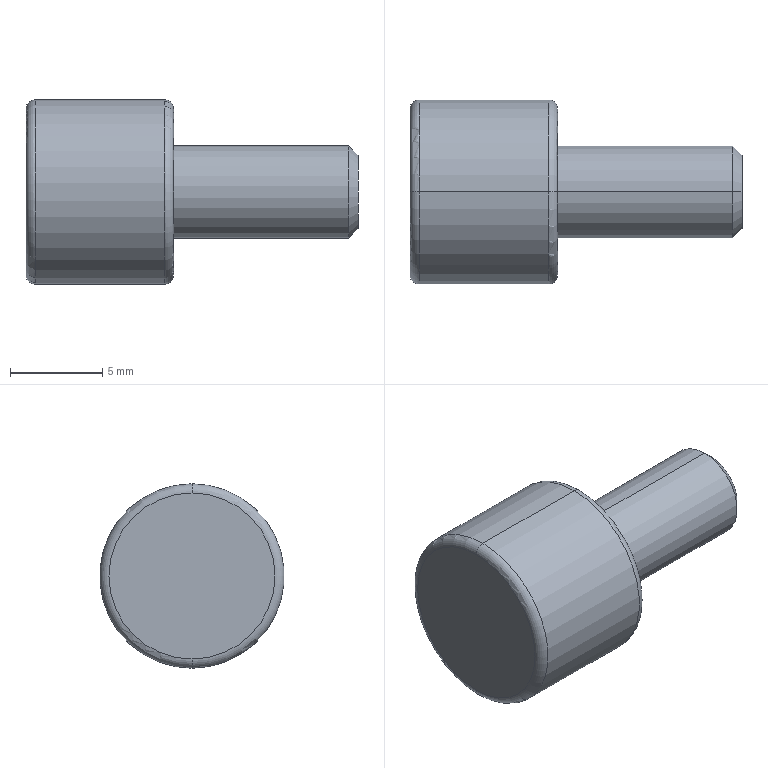Part | STEP file | CFFANG5-10_デフォルト | 1 solid | 13 faces | box 18 x 10 x 10 mm | volume 819.54 mm3 | torus 4 | cylinder 4 | plane 3 | cone 2 | commonest cylinder face diameters 5 x2 10 x2
STEP:
#1=CARTESIAN_POINT('',(18.,0.,-2.));
#2=VERTEX_POINT('',#1);
#3=CARTESIAN_POINT('',(18.,0.,2.));
#4=VERTEX_POINT('',#3);
#5=CARTESIAN_POINT('',(18.,0.,0.));
#6=DIRECTION('',(1.,0.,0.));
#7=DIRECTION('',(0.,0.,1.));
#8=AXIS2_PLACEMENT_3D('',#5,#6,#7);
#9=CIRCLE('',#8,2.);
#10=EDGE_CURVE('',#2,#4,#9,.T.);
#11=ORIENTED_EDGE('',*,*,#10,.F.);
#12=CARTESIAN_POINT('',(17.5,0.,-2.5));
#13=VERTEX_POINT('',#12);
#14=CARTESIAN_POINT('',(17.5,0.,-2.5));
#15=DIRECTION('',(-0.7071,0.,-0.7071));
#16=VECTOR('',#15,1000.);
#17=LINE('',#14,#16);
#18=EDGE_CURVE('',#2,#13,#17,.T.);
#19=ORIENTED_EDGE('',*,*,#18,.T.);
#20=CARTESIAN_POINT('',(17.5,0.,2.5));
#21=VERTEX_POINT('',#20);
#22=CARTESIAN_POINT('',(17.5,0.,0.));
#23=DIRECTION('',(-1.,0.,0.));
#24=DIRECTION('',(0.,0.,1.));
#25=AXIS2_PLACEMENT_3D('',#22,#23,#24);
#26=CIRCLE('',#25,2.5);
#27=EDGE_CURVE('',#21,#13,#26,.T.);
#28=ORIENTED_EDGE('',*,*,#27,.F.);
#29=CARTESIAN_POINT('',(17.5,0.,2.5));
#30=DIRECTION('',(-0.7071,0.,0.7071));
#31=VECTOR('',#30,1000.);
#32=LINE('',#29,#31);
#33=EDGE_CURVE('',#4,#21,#32,.T.);
#34=ORIENTED_EDGE('',*,*,#33,.F.);
#35=EDGE_LOOP('',(#11,#19,#28,#34));
#36=FACE_OUTER_BOUND('',#35,.T.);
#37=CARTESIAN_POINT('',(17.5,0.,0.));
#38=DIRECTION('',(-1.,0.,0.));
#39=DIRECTION('',(0.,0.,1.));
#40=AXIS2_PLACEMENT_3D('',#37,#38,#39);
#41=CONICAL_SURFACE('',#40,2.5,0.7854);
#42=ADVANCED_FACE('',(#36),#41,.T.);
#43=CARTESIAN_POINT('',(0.,0.,4.5));
#44=VERTEX_POINT('',#43);
#45=CARTESIAN_POINT('',(0.,0.,-4.5));
#46=VERTEX_POINT('',#45);
#47=CARTESIAN_POINT('',(0.,0.,0.));
#48=DIRECTION('',(-1.,0.,0.));
#49=DIRECTION('',(0.,0.,-1.));
#50=AXIS2_PLACEMENT_3D('',#47,#48,#49);
#51=CIRCLE('',#50,4.5);
#52=EDGE_CURVE('',#44,#46,#51,.T.);
#53=ORIENTED_EDGE('',*,*,#52,.F.);
#54=CARTESIAN_POINT('',(0.5,0.,5.));
#55=VERTEX_POINT('',#54);
#56=CARTESIAN_POINT('',(0.5,0.,4.5));
#57=DIRECTION('',(0.,1.,0.));
#58=DIRECTION('',(0.,0.,1.));
#59=AXIS2_PLACEMENT_3D('',#56,#57,#58);
#60=CIRCLE('',#59,0.5);
#61=EDGE_CURVE('',#44,#55,#60,.T.);
#62=ORIENTED_EDGE('',*,*,#61,.T.);
#63=CARTESIAN_POINT('',(0.5,0.,-5.));
#64=VERTEX_POINT('',#63);
#65=CARTESIAN_POINT('',(0.5,0.,0.));
#66=DIRECTION('',(1.,0.,0.));
#67=DIRECTION('',(0.,0.,-1.));
#68=AXIS2_PLACEMENT_3D('',#65,#66,#67);
#69=CIRCLE('',#68,5.);
#70=EDGE_CURVE('',#64,#55,#69,.T.);
#71=ORIENTED_EDGE('',*,*,#70,.F.);
#72=CARTESIAN_POINT('',(0.5,0.,-4.5));
#73=DIRECTION('',(0.,-1.,0.));
#74=DIRECTION('',(0.,0.,-1.));
#75=AXIS2_PLACEMENT_3D('',#72,#73,#74);
#76=CIRCLE('',#75,0.5);
#77=EDGE_CURVE('',#46,#64,#76,.T.);
#78=ORIENTED_EDGE('',*,*,#77,.F.);
#79=EDGE_LOOP('',(#53,#62,#71,#78));
#80=FACE_OUTER_BOUND('',#79,.T.);
#81=CARTESIAN_POINT('',(0.5,0.,0.));
#82=DIRECTION('',(1.,0.,0.));
#83=DIRECTION('',(0.,0.,-1.));
#84=AXIS2_PLACEMENT_3D('',#81,#82,#83);
#85=TOROIDAL_SURFACE('',#84,4.5,0.5);
#86=ADVANCED_FACE('',(#80),#85,.T.);
#87=CARTESIAN_POINT('',(8.,0.,-4.5));
#88=VERTEX_POINT('',#87);
#89=CARTESIAN_POINT('',(8.,0.,4.5));
#90=VERTEX_POINT('',#89);
#91=CARTESIAN_POINT('',(8.,0.,0.));
#92=DIRECTION('',(1.,0.,0.));
#93=DIRECTION('',(0.,0.,1.));
#94=AXIS2_PLACEMENT_3D('',#91,#92,#93);
#95=CIRCLE('',#94,4.5);
#96=EDGE_CURVE('',#88,#90,#95,.T.);
#97=ORIENTED_EDGE('',*,*,#96,.F.);
#98=CARTESIAN_POINT('',(7.5,0.,-5.));
#99=VERTEX_POINT('',#98);
#100=CARTESIAN_POINT('',(7.5,0.,-4.5));
#101=DIRECTION('',(0.,1.,0.));
#102=DIRECTION('',(0.,0.,1.));
#103=AXIS2_PLACEMENT_3D('',#100,#101,#102);
#104=CIRCLE('',#103,0.5);
#105=EDGE_CURVE('',#88,#99,#104,.T.);
#106=ORIENTED_EDGE('',*,*,#105,.T.);
#107=CARTESIAN_POINT('',(7.5,0.,5.));
#108=VERTEX_POINT('',#107);
#109=CARTESIAN_POINT('',(7.5,0.,0.));
#110=DIRECTION('',(-1.,0.,0.));
#111=DIRECTION('',(0.,0.,1.));
#112=AXIS2_PLACEMENT_3D('',#109,#110,#111);
#113=CIRCLE('',#112,5.);
#114=EDGE_CURVE('',#108,#99,#113,.T.);
#115=ORIENTED_EDGE('',*,*,#114,.F.);
#116=CARTESIAN_POINT('',(7.5,0.,4.5));
#117=DIRECTION('',(0.,-1.,0.));
#118=DIRECTION('',(0.,0.,-1.));
#119=AXIS2_PLACEMENT_3D('',#116,#117,#118);
#120=CIRCLE('',#119,0.5);
#121=EDGE_CURVE('',#90,#108,#120,.T.);
#122=ORIENTED_EDGE('',*,*,#121,.F.);
#123=EDGE_LOOP('',(#97,#106,#115,#122));
#124=FACE_OUTER_BOUND('',#123,.T.);
#125=CARTESIAN_POINT('',(7.5,0.,0.));
#126=DIRECTION('',(-1.,0.,0.));
#127=DIRECTION('',(0.,0.,1.));
#128=AXIS2_PLACEMENT_3D('',#125,#126,#127);
#129=TOROIDAL_SURFACE('',#128,4.5,0.5);
#130=ADVANCED_FACE('',(#124),#129,.T.);
#131=ORIENTED_EDGE('',*,*,#27,.T.);
#132=CARTESIAN_POINT('',(8.,0.,-2.5));
#133=VERTEX_POINT('',#132);
#134=CARTESIAN_POINT('',(0.,0.,-2.5));
#135=DIRECTION('',(-1.,0.,0.));
#136=VECTOR('',#135,1000.);
#137=LINE('',#134,#136);
#138=EDGE_CURVE('',#13,#133,#137,.T.);
#139=ORIENTED_EDGE('',*,*,#138,.T.);
#140=CARTESIAN_POINT('',(8.,0.,2.5));
#141=VERTEX_POINT('',#140);
#142=CARTESIAN_POINT('',(8.,0.,0.));
#143=DIRECTION('',(-1.,0.,0.));
#144=DIRECTION('',(0.,0.,1.));
#145=AXIS2_PLACEMENT_3D('',#142,#143,#144);
#146=CIRCLE('',#145,2.5);
#147=EDGE_CURVE('',#141,#133,#146,.T.);
#148=ORIENTED_EDGE('',*,*,#147,.F.);
#149=CARTESIAN_POINT('',(0.,0.,2.5));
#150=DIRECTION('',(-1.,0.,0.));
#151=VECTOR('',#150,1000.);
#152=LINE('',#149,#151);
#153=EDGE_CURVE('',#21,#141,#152,.T.);
#154=ORIENTED_EDGE('',*,*,#153,.F.);
#155=EDGE_LOOP('',(#131,#139,#148,#154));
#156=FACE_OUTER_BOUND('',#155,.T.);
#157=CARTESIAN_POINT('',(0.,0.,0.));
#158=DIRECTION('',(-1.,0.,0.));
#159=DIRECTION('',(0.,0.,1.));
#160=AXIS2_PLACEMENT_3D('',#157,#158,#159);
#161=CYLINDRICAL_SURFACE('',#160,2.5);
#162=ADVANCED_FACE('',(#156),#161,.T.);
#163=ORIENTED_EDGE('',*,*,#114,.T.);
#164=CARTESIAN_POINT('',(0.,0.,-5.));
#165=DIRECTION('',(-1.,0.,0.));
#166=VECTOR('',#165,1000.);
#167=LINE('',#164,#166);
#168=EDGE_CURVE('',#99,#64,#167,.T.);
#169=ORIENTED_EDGE('',*,*,#168,.T.);
#170=ORIENTED_EDGE('',*,*,#70,.T.);
#171=CARTESIAN_POINT('',(0.,0.,5.));
#172=DIRECTION('',(-1.,0.,0.));
#173=VECTOR('',#172,1000.);
#174=LINE('',#171,#173);
#175=EDGE_CURVE('',#108,#55,#174,.T.);
#176=ORIENTED_EDGE('',*,*,#175,.F.);
#177=EDGE_LOOP('',(#163,#169,#170,#176));
#178=FACE_OUTER_BOUND('',#177,.T.);
#179=CARTESIAN_POINT('',(0.,0.,0.));
#180=DIRECTION('',(-1.,0.,0.));
#181=DIRECTION('',(0.,0.,1.));
#182=AXIS2_PLACEMENT_3D('',#179,#180,#181);
#183=CYLINDRICAL_SURFACE('',#182,5.);
#184=ADVANCED_FACE('',(#178),#183,.T.);
#185=CARTESIAN_POINT('',(0.,0.,0.));
#186=DIRECTION('',(-1.,0.,0.));
#187=DIRECTION('',(0.,0.,-1.));
#188=AXIS2_PLACEMENT_3D('',#185,#186,#187);
#189=CIRCLE('',#188,4.5);
#190=EDGE_CURVE('',#46,#44,#189,.T.);
#191=ORIENTED_EDGE('',*,*,#190,.T.);
#192=ORIENTED_EDGE('',*,*,#52,.T.);
#193=EDGE_LOOP('',(#191,#192));
#194=FACE_OUTER_BOUND('',#193,.T.);
#195=CARTESIAN_POINT('',(0.,0.,0.));
#196=DIRECTION('',(1.,0.,0.));
#197=DIRECTION('',(0.,0.,-1.));
#198=AXIS2_PLACEMENT_3D('',#195,#196,#197);
#199=PLANE('',#198);
#200=ADVANCED_FACE('',(#194),#199,.F.);
#201=ORIENTED_EDGE('',*,*,#168,.F.);
#202=CARTESIAN_POINT('',(7.5,0.,0.));
#203=DIRECTION('',(-1.,0.,0.));
#204=DIRECTION('',(0.,0.,1.));
#205=AXIS2_PLACEMENT_3D('',#202,#203,#204);
#206=CIRCLE('',#205,5.);
#207=EDGE_CURVE('',#99,#108,#206,.T.);
#208=ORIENTED_EDGE('',*,*,#207,.T.);
#209=ORIENTED_EDGE('',*,*,#175,.T.);
#210=CARTESIAN_POINT('',(0.5,0.,0.));
#211=DIRECTION('',(1.,0.,0.));
#212=DIRECTION('',(0.,0.,-1.));
#213=AXIS2_PLACEMENT_3D('',#210,#211,#212);
#214=CIRCLE('',#213,5.);
#215=EDGE_CURVE('',#55,#64,#214,.T.);
#216=ORIENTED_EDGE('',*,*,#215,.T.);
#217=EDGE_LOOP('',(#201,#208,#209,#216));
#218=FACE_OUTER_BOUND('',#217,.T.);
#219=CARTESIAN_POINT('',(0.,0.,0.));
#220=DIRECTION('',(-1.,0.,0.));
#221=DIRECTION('',(0.,0.,1.));
#222=AXIS2_PLACEMENT_3D('',#219,#220,#221);
#223=CYLINDRICAL_SURFACE('',#222,5.);
#224=ADVANCED_FACE('',(#218),#223,.T.);
#225=CARTESIAN_POINT('',(8.,0.,0.));
#226=DIRECTION('',(1.,0.,0.));
#227=DIRECTION('',(0.,0.,1.));
#228=AXIS2_PLACEMENT_3D('',#225,#226,#227);
#229=CIRCLE('',#228,4.5);
#230=EDGE_CURVE('',#90,#88,#229,.T.);
#231=ORIENTED_EDGE('',*,*,#230,.T.);
#232=ORIENTED_EDGE('',*,*,#96,.T.);
#233=EDGE_LOOP('',(#231,#232));
#234=FACE_OUTER_BOUND('',#233,.T.);
#235=ORIENTED_EDGE('',*,*,#147,.T.);
#236=CARTESIAN_POINT('',(8.,0.,0.));
#237=DIRECTION('',(-1.,0.,0.));
#238=DIRECTION('',(0.,0.,1.));
#239=AXIS2_PLACEMENT_3D('',#236,#237,#238);
#240=CIRCLE('',#239,2.5);
#241=EDGE_CURVE('',#133,#141,#240,.T.);
#242=ORIENTED_EDGE('',*,*,#241,.T.);
#243=EDGE_LOOP('',(#235,#242));
#244=FACE_BOUND('',#243,.T.);
#245=CARTESIAN_POINT('',(8.,5.,0.));
#246=DIRECTION('',(-1.,0.,0.));
#247=DIRECTION('',(0.,0.,1.));
#248=AXIS2_PLACEMENT_3D('',#245,#246,#247);
#249=PLANE('',#248);
#250=ADVANCED_FACE('',(#234,#244),#249,.F.);
#251=ORIENTED_EDGE('',*,*,#138,.F.);
#252=CARTESIAN_POINT('',(17.5,0.,0.));
#253=DIRECTION('',(-1.,0.,0.));
#254=DIRECTION('',(0.,0.,1.));
#255=AXIS2_PLACEMENT_3D('',#252,#253,#254);
#256=CIRCLE('',#255,2.5);
#257=EDGE_CURVE('',#13,#21,#256,.T.);
#258=ORIENTED_EDGE('',*,*,#257,.T.);
#259=ORIENTED_EDGE('',*,*,#153,.T.);
#260=ORIENTED_EDGE('',*,*,#241,.F.);
#261=EDGE_LOOP('',(#251,#258,#259,#260));
#262=FACE_OUTER_BOUND('',#261,.T.);
#263=CARTESIAN_POINT('',(0.,0.,0.));
#264=DIRECTION('',(-1.,0.,0.));
#265=DIRECTION('',(0.,0.,1.));
#266=AXIS2_PLACEMENT_3D('',#263,#264,#265);
#267=CYLINDRICAL_SURFACE('',#266,2.5);
#268=ADVANCED_FACE('',(#262),#267,.T.);
#269=CARTESIAN_POINT('',(18.,0.,0.));
#270=DIRECTION('',(1.,0.,0.));
#271=DIRECTION('',(0.,0.,1.));
#272=AXIS2_PLACEMENT_3D('',#269,#270,#271);
#273=CIRCLE('',#272,2.);
#274=EDGE_CURVE('',#4,#2,#273,.T.);
#275=ORIENTED_EDGE('',*,*,#274,.T.);
#276=ORIENTED_EDGE('',*,*,#10,.T.);
#277=EDGE_LOOP('',(#275,#276));
#278=FACE_OUTER_BOUND('',#277,.T.);
#279=CARTESIAN_POINT('',(18.,2.5,0.));
#280=DIRECTION('',(-1.,0.,0.));
#281=DIRECTION('',(0.,0.,1.));
#282=AXIS2_PLACEMENT_3D('',#279,#280,#281);
#283=PLANE('',#282);
#284=ADVANCED_FACE('',(#278),#283,.F.);
#285=ORIENTED_EDGE('',*,*,#105,.F.);
#286=ORIENTED_EDGE('',*,*,#230,.F.);
#287=ORIENTED_EDGE('',*,*,#121,.T.);
#288=ORIENTED_EDGE('',*,*,#207,.F.);
#289=EDGE_LOOP('',(#285,#286,#287,#288));
#290=FACE_OUTER_BOUND('',#289,.T.);
#291=CARTESIAN_POINT('',(7.5,0.,0.));
#292=DIRECTION('',(-1.,0.,0.));
#293=DIRECTION('',(0.,0.,1.));
#294=AXIS2_PLACEMENT_3D('',#291,#292,#293);
#295=TOROIDAL_SURFACE('',#294,4.5,0.5);
#296=ADVANCED_FACE('',(#290),#295,.T.);
#297=ORIENTED_EDGE('',*,*,#61,.F.);
#298=ORIENTED_EDGE('',*,*,#190,.F.);
#299=ORIENTED_EDGE('',*,*,#77,.T.);
#300=ORIENTED_EDGE('',*,*,#215,.F.);
#301=EDGE_LOOP('',(#297,#298,#299,#300));
#302=FACE_OUTER_BOUND('',#301,.T.);
#303=CARTESIAN_POINT('',(0.5,0.,0.));
#304=DIRECTION('',(1.,0.,0.));
#305=DIRECTION('',(0.,0.,-1.));
#306=AXIS2_PLACEMENT_3D('',#303,#304,#305);
#307=TOROIDAL_SURFACE('',#306,4.5,0.5);
#308=ADVANCED_FACE('',(#302),#307,.T.);
#309=ORIENTED_EDGE('',*,*,#18,.F.);
#310=ORIENTED_EDGE('',*,*,#274,.F.);
#311=ORIENTED_EDGE('',*,*,#33,.T.);
#312=ORIENTED_EDGE('',*,*,#257,.F.);
#313=EDGE_LOOP('',(#309,#310,#311,#312));
#314=FACE_OUTER_BOUND('',#313,.T.);
#315=CARTESIAN_POINT('',(17.5,0.,0.));
#316=DIRECTION('',(-1.,0.,0.));
#317=DIRECTION('',(0.,0.,1.));
#318=AXIS2_PLACEMENT_3D('',#315,#316,#317);
#319=CONICAL_SURFACE('',#318,2.5,0.7854);
#320=ADVANCED_FACE('',(#314),#319,.T.);
#321=CLOSED_SHELL('',(#42,#86,#130,#162,#184,#200,#224,#250,#268,#284,#296,#308,#320));
#322=MANIFOLD_SOLID_BREP('',#321);
#323=CARTESIAN_POINT('',(0.,0.,0.));
#324=DIRECTION('',(0.,0.,1.));
#325=DIRECTION('',(1.,0.,0.));
#326=AXIS2_PLACEMENT_3D('',#323,#324,#325);
#327=(LENGTH_UNIT()NAMED_UNIT(*)SI_UNIT(.MILLI.,.METRE.));
#328=UNCERTAINTY_MEASURE_WITH_UNIT(LENGTH_MEASURE(0.00001),#327,'','');
#329=(NAMED_UNIT(*)PLANE_ANGLE_UNIT()SI_UNIT($,.RADIAN.));
#330=(NAMED_UNIT(*)SI_UNIT($,.STERADIAN.)SOLID_ANGLE_UNIT());
#331=(GEOMETRIC_REPRESENTATION_CONTEXT(3)GLOBAL_UNCERTAINTY_ASSIGNED_CONTEXT((#328))GLOBAL_UNIT_ASSIGNED_CONTEXT((#327,#329,#330))REPRESENTATION_CONTEXT('',''));
#332=ADVANCED_BREP_SHAPE_REPRESENTATION('',(#322,#326),#331);